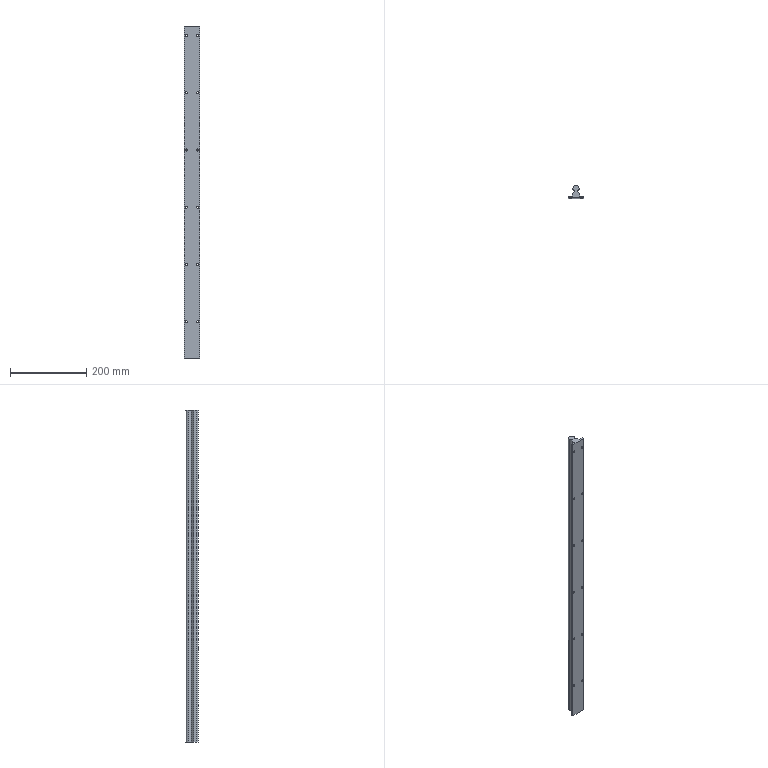Part | SolidWorks | features Extrusion 1, HoleWzd 1, ICE 1, LPattern 1 | 1 solid | 42 faces | box 40 x 33 x 870 mm | volume 521685 mm3 | cylinder 27 | plane 15 | commonest cylinder face diameters 5.5 x24 16 x3
STEP:
#1=CARTESIAN_POINT('',(15.,0.,-342.75));
#2=VERTEX_POINT('',#1);
#3=CARTESIAN_POINT('',(15.,0.,-337.25));
#4=VERTEX_POINT('',#3);
#5=CARTESIAN_POINT('',(15.,0.,-340.));
#6=DIRECTION('',(0.,1.,0.));
#7=DIRECTION('',(0.,0.,1.));
#8=AXIS2_PLACEMENT_3D('',#5,#6,#7);
#9=CIRCLE('',#8,2.75);
#10=EDGE_CURVE('',#2,#4,#9,.T.);
#11=ORIENTED_EDGE('',*,*,#10,.F.);
#12=CARTESIAN_POINT('',(15.,5.,-342.75));
#13=VERTEX_POINT('',#12);
#14=CARTESIAN_POINT('',(15.,5.,-342.75));
#15=DIRECTION('',(0.,1.,0.));
#16=VECTOR('',#15,1000.);
#17=LINE('',#14,#16);
#18=EDGE_CURVE('',#2,#13,#17,.T.);
#19=ORIENTED_EDGE('',*,*,#18,.T.);
#20=CARTESIAN_POINT('',(15.,5.,-337.25));
#21=VERTEX_POINT('',#20);
#22=CARTESIAN_POINT('',(15.,5.,-340.));
#23=DIRECTION('',(0.,1.,0.));
#24=DIRECTION('',(0.,0.,1.));
#25=AXIS2_PLACEMENT_3D('',#22,#23,#24);
#26=CIRCLE('',#25,2.75);
#27=EDGE_CURVE('',#13,#21,#26,.T.);
#28=ORIENTED_EDGE('',*,*,#27,.T.);
#29=CARTESIAN_POINT('',(15.,5.,-337.25));
#30=DIRECTION('',(0.,1.,0.));
#31=VECTOR('',#30,1000.);
#32=LINE('',#29,#31);
#33=EDGE_CURVE('',#4,#21,#32,.T.);
#34=ORIENTED_EDGE('',*,*,#33,.F.);
#35=EDGE_LOOP('',(#11,#19,#28,#34));
#36=FACE_OUTER_BOUND('',#35,.T.);
#37=CARTESIAN_POINT('',(15.,5.,-340.));
#38=DIRECTION('',(0.,1.,0.));
#39=DIRECTION('',(0.,0.,1.));
#40=AXIS2_PLACEMENT_3D('',#37,#38,#39);
#41=CYLINDRICAL_SURFACE('',#40,2.75);
#42=ADVANCED_FACE('',(#36),#41,.F.);
#43=CARTESIAN_POINT('',(-15.,0.,-342.75));
#44=VERTEX_POINT('',#43);
#45=CARTESIAN_POINT('',(-15.,0.,-337.25));
#46=VERTEX_POINT('',#45);
#47=CARTESIAN_POINT('',(-15.,0.,-340.));
#48=DIRECTION('',(0.,1.,0.));
#49=DIRECTION('',(0.,0.,1.));
#50=AXIS2_PLACEMENT_3D('',#47,#48,#49);
#51=CIRCLE('',#50,2.75);
#52=EDGE_CURVE('',#44,#46,#51,.T.);
#53=ORIENTED_EDGE('',*,*,#52,.F.);
#54=CARTESIAN_POINT('',(-15.,5.,-342.75));
#55=VERTEX_POINT('',#54);
#56=CARTESIAN_POINT('',(-15.,5.,-342.75));
#57=DIRECTION('',(0.,1.,0.));
#58=VECTOR('',#57,1000.);
#59=LINE('',#56,#58);
#60=EDGE_CURVE('',#44,#55,#59,.T.);
#61=ORIENTED_EDGE('',*,*,#60,.T.);
#62=CARTESIAN_POINT('',(-15.,5.,-337.25));
#63=VERTEX_POINT('',#62);
#64=CARTESIAN_POINT('',(-15.,5.,-340.));
#65=DIRECTION('',(0.,1.,0.));
#66=DIRECTION('',(0.,0.,1.));
#67=AXIS2_PLACEMENT_3D('',#64,#65,#66);
#68=CIRCLE('',#67,2.75);
#69=EDGE_CURVE('',#55,#63,#68,.T.);
#70=ORIENTED_EDGE('',*,*,#69,.T.);
#71=CARTESIAN_POINT('',(-15.,5.,-337.25));
#72=DIRECTION('',(0.,1.,0.));
#73=VECTOR('',#72,1000.);
#74=LINE('',#71,#73);
#75=EDGE_CURVE('',#46,#63,#74,.T.);
#76=ORIENTED_EDGE('',*,*,#75,.F.);
#77=EDGE_LOOP('',(#53,#61,#70,#76));
#78=FACE_OUTER_BOUND('',#77,.T.);
#79=CARTESIAN_POINT('',(-15.,5.,-340.));
#80=DIRECTION('',(0.,1.,0.));
#81=DIRECTION('',(0.,0.,1.));
#82=AXIS2_PLACEMENT_3D('',#79,#80,#81);
#83=CYLINDRICAL_SURFACE('',#82,2.75);
#84=ADVANCED_FACE('',(#78),#83,.F.);
#85=CARTESIAN_POINT('',(15.,0.,-192.75));
#86=VERTEX_POINT('',#85);
#87=CARTESIAN_POINT('',(15.,0.,-187.25));
#88=VERTEX_POINT('',#87);
#89=CARTESIAN_POINT('',(15.,0.,-190.));
#90=DIRECTION('',(0.,1.,0.));
#91=DIRECTION('',(0.,0.,1.));
#92=AXIS2_PLACEMENT_3D('',#89,#90,#91);
#93=CIRCLE('',#92,2.75);
#94=EDGE_CURVE('',#86,#88,#93,.T.);
#95=ORIENTED_EDGE('',*,*,#94,.F.);
#96=CARTESIAN_POINT('',(15.,5.,-192.75));
#97=VERTEX_POINT('',#96);
#98=CARTESIAN_POINT('',(15.,5.,-192.75));
#99=DIRECTION('',(0.,1.,0.));
#100=VECTOR('',#99,1000.);
#101=LINE('',#98,#100);
#102=EDGE_CURVE('',#86,#97,#101,.T.);
#103=ORIENTED_EDGE('',*,*,#102,.T.);
#104=CARTESIAN_POINT('',(15.,5.,-187.25));
#105=VERTEX_POINT('',#104);
#106=CARTESIAN_POINT('',(15.,5.,-190.));
#107=DIRECTION('',(0.,1.,0.));
#108=DIRECTION('',(0.,0.,1.));
#109=AXIS2_PLACEMENT_3D('',#106,#107,#108);
#110=CIRCLE('',#109,2.75);
#111=EDGE_CURVE('',#97,#105,#110,.T.);
#112=ORIENTED_EDGE('',*,*,#111,.T.);
#113=CARTESIAN_POINT('',(15.,5.,-187.25));
#114=DIRECTION('',(0.,1.,0.));
#115=VECTOR('',#114,1000.);
#116=LINE('',#113,#115);
#117=EDGE_CURVE('',#88,#105,#116,.T.);
#118=ORIENTED_EDGE('',*,*,#117,.F.);
#119=EDGE_LOOP('',(#95,#103,#112,#118));
#120=FACE_OUTER_BOUND('',#119,.T.);
#121=CARTESIAN_POINT('',(15.,5.,-190.));
#122=DIRECTION('',(0.,1.,0.));
#123=DIRECTION('',(0.,0.,1.));
#124=AXIS2_PLACEMENT_3D('',#121,#122,#123);
#125=CYLINDRICAL_SURFACE('',#124,2.75);
#126=ADVANCED_FACE('',(#120),#125,.F.);
#127=CARTESIAN_POINT('',(-15.,0.,-192.75));
#128=VERTEX_POINT('',#127);
#129=CARTESIAN_POINT('',(-15.,0.,-187.25));
#130=VERTEX_POINT('',#129);
#131=CARTESIAN_POINT('',(-15.,0.,-190.));
#132=DIRECTION('',(0.,1.,0.));
#133=DIRECTION('',(0.,0.,1.));
#134=AXIS2_PLACEMENT_3D('',#131,#132,#133);
#135=CIRCLE('',#134,2.75);
#136=EDGE_CURVE('',#128,#130,#135,.T.);
#137=ORIENTED_EDGE('',*,*,#136,.F.);
#138=CARTESIAN_POINT('',(-15.,5.,-192.75));
#139=VERTEX_POINT('',#138);
#140=CARTESIAN_POINT('',(-15.,5.,-192.75));
#141=DIRECTION('',(0.,1.,0.));
#142=VECTOR('',#141,1000.);
#143=LINE('',#140,#142);
#144=EDGE_CURVE('',#128,#139,#143,.T.);
#145=ORIENTED_EDGE('',*,*,#144,.T.);
#146=CARTESIAN_POINT('',(-15.,5.,-187.25));
#147=VERTEX_POINT('',#146);
#148=CARTESIAN_POINT('',(-15.,5.,-190.));
#149=DIRECTION('',(0.,1.,0.));
#150=DIRECTION('',(0.,0.,1.));
#151=AXIS2_PLACEMENT_3D('',#148,#149,#150);
#152=CIRCLE('',#151,2.75);
#153=EDGE_CURVE('',#139,#147,#152,.T.);
#154=ORIENTED_EDGE('',*,*,#153,.T.);
#155=CARTESIAN_POINT('',(-15.,5.,-187.25));
#156=DIRECTION('',(0.,1.,0.));
#157=VECTOR('',#156,1000.);
#158=LINE('',#155,#157);
#159=EDGE_CURVE('',#130,#147,#158,.T.);
#160=ORIENTED_EDGE('',*,*,#159,.F.);
#161=EDGE_LOOP('',(#137,#145,#154,#160));
#162=FACE_OUTER_BOUND('',#161,.T.);
#163=CARTESIAN_POINT('',(-15.,5.,-190.));
#164=DIRECTION('',(0.,1.,0.));
#165=DIRECTION('',(0.,0.,1.));
#166=AXIS2_PLACEMENT_3D('',#163,#164,#165);
#167=CYLINDRICAL_SURFACE('',#166,2.75);
#168=ADVANCED_FACE('',(#162),#167,.F.);
#169=CARTESIAN_POINT('',(15.,0.,-42.75));
#170=VERTEX_POINT('',#169);
#171=CARTESIAN_POINT('',(15.,0.,-37.25));
#172=VERTEX_POINT('',#171);
#173=CARTESIAN_POINT('',(15.,0.,-40.));
#174=DIRECTION('',(0.,1.,0.));
#175=DIRECTION('',(0.,0.,1.));
#176=AXIS2_PLACEMENT_3D('',#173,#174,#175);
#177=CIRCLE('',#176,2.75);
#178=EDGE_CURVE('',#170,#172,#177,.T.);
#179=ORIENTED_EDGE('',*,*,#178,.F.);
#180=CARTESIAN_POINT('',(15.,5.,-42.75));
#181=VERTEX_POINT('',#180);
#182=CARTESIAN_POINT('',(15.,5.,-42.75));
#183=DIRECTION('',(0.,1.,0.));
#184=VECTOR('',#183,1000.);
#185=LINE('',#182,#184);
#186=EDGE_CURVE('',#170,#181,#185,.T.);
#187=ORIENTED_EDGE('',*,*,#186,.T.);
#188=CARTESIAN_POINT('',(15.,5.,-37.25));
#189=VERTEX_POINT('',#188);
#190=CARTESIAN_POINT('',(15.,5.,-40.));
#191=DIRECTION('',(0.,1.,0.));
#192=DIRECTION('',(0.,0.,1.));
#193=AXIS2_PLACEMENT_3D('',#190,#191,#192);
#194=CIRCLE('',#193,2.75);
#195=EDGE_CURVE('',#181,#189,#194,.T.);
#196=ORIENTED_EDGE('',*,*,#195,.T.);
#197=CARTESIAN_POINT('',(15.,5.,-37.25));
#198=DIRECTION('',(0.,1.,0.));
#199=VECTOR('',#198,1000.);
#200=LINE('',#197,#199);
#201=EDGE_CURVE('',#172,#189,#200,.T.);
#202=ORIENTED_EDGE('',*,*,#201,.F.);
#203=EDGE_LOOP('',(#179,#187,#196,#202));
#204=FACE_OUTER_BOUND('',#203,.T.);
#205=CARTESIAN_POINT('',(15.,5.,-40.));
#206=DIRECTION('',(0.,1.,0.));
#207=DIRECTION('',(0.,0.,1.));
#208=AXIS2_PLACEMENT_3D('',#205,#206,#207);
#209=CYLINDRICAL_SURFACE('',#208,2.75);
#210=ADVANCED_FACE('',(#204),#209,.F.);
#211=CARTESIAN_POINT('',(-15.,0.,-42.75));
#212=VERTEX_POINT('',#211);
#213=CARTESIAN_POINT('',(-15.,0.,-37.25));
#214=VERTEX_POINT('',#213);
#215=CARTESIAN_POINT('',(-15.,0.,-40.));
#216=DIRECTION('',(0.,1.,0.));
#217=DIRECTION('',(0.,0.,1.));
#218=AXIS2_PLACEMENT_3D('',#215,#216,#217);
#219=CIRCLE('',#218,2.75);
#220=EDGE_CURVE('',#212,#214,#219,.T.);
#221=ORIENTED_EDGE('',*,*,#220,.F.);
#222=CARTESIAN_POINT('',(-15.,5.,-42.75));
#223=VERTEX_POINT('',#222);
#224=CARTESIAN_POINT('',(-15.,5.,-42.75));
#225=DIRECTION('',(0.,1.,0.));
#226=VECTOR('',#225,1000.);
#227=LINE('',#224,#226);
#228=EDGE_CURVE('',#212,#223,#227,.T.);
#229=ORIENTED_EDGE('',*,*,#228,.T.);
#230=CARTESIAN_POINT('',(-15.,5.,-37.25));
#231=VERTEX_POINT('',#230);
#232=CARTESIAN_POINT('',(-15.,5.,-40.));
#233=DIRECTION('',(0.,1.,0.));
#234=DIRECTION('',(0.,0.,1.));
#235=AXIS2_PLACEMENT_3D('',#232,#233,#234);
#236=CIRCLE('',#235,2.75);
#237=EDGE_CURVE('',#223,#231,#236,.T.);
#238=ORIENTED_EDGE('',*,*,#237,.T.);
#239=CARTESIAN_POINT('',(-15.,5.,-37.25));
#240=DIRECTION('',(0.,1.,0.));
#241=VECTOR('',#240,1000.);
#242=LINE('',#239,#241);
#243=EDGE_CURVE('',#214,#231,#242,.T.);
#244=ORIENTED_EDGE('',*,*,#243,.F.);
#245=EDGE_LOOP('',(#221,#229,#238,#244));
#246=FACE_OUTER_BOUND('',#245,.T.);
#247=CARTESIAN_POINT('',(-15.,5.,-40.));
#248=DIRECTION('',(0.,1.,0.));
#249=DIRECTION('',(0.,0.,1.));
#250=AXIS2_PLACEMENT_3D('',#247,#248,#249);
#251=CYLINDRICAL_SURFACE('',#250,2.75);
#252=ADVANCED_FACE('',(#246),#251,.F.);
#253=CARTESIAN_POINT('',(15.,0.,107.25));
#254=VERTEX_POINT('',#253);
#255=CARTESIAN_POINT('',(15.,0.,112.75));
#256=VERTEX_POINT('',#255);
#257=CARTESIAN_POINT('',(15.,0.,110.));
#258=DIRECTION('',(0.,1.,0.));
#259=DIRECTION('',(0.,0.,1.));
#260=AXIS2_PLACEMENT_3D('',#257,#258,#259);
#261=CIRCLE('',#260,2.75);
#262=EDGE_CURVE('',#254,#256,#261,.T.);
#263=ORIENTED_EDGE('',*,*,#262,.F.);
#264=CARTESIAN_POINT('',(15.,5.,107.25));
#265=VERTEX_POINT('',#264);
#266=CARTESIAN_POINT('',(15.,5.,107.25));
#267=DIRECTION('',(0.,1.,0.));
#268=VECTOR('',#267,1000.);
#269=LINE('',#266,#268);
#270=EDGE_CURVE('',#254,#265,#269,.T.);
#271=ORIENTED_EDGE('',*,*,#270,.T.);
#272=CARTESIAN_POINT('',(15.,5.,112.75));
#273=VERTEX_POINT('',#272);
#274=CARTESIAN_POINT('',(15.,5.,110.));
#275=DIRECTION('',(0.,1.,0.));
#276=DIRECTION('',(0.,0.,1.));
#277=AXIS2_PLACEMENT_3D('',#274,#275,#276);
#278=CIRCLE('',#277,2.75);
#279=EDGE_CURVE('',#265,#273,#278,.T.);
#280=ORIENTED_EDGE('',*,*,#279,.T.);
#281=CARTESIAN_POINT('',(15.,5.,112.75));
#282=DIRECTION('',(0.,1.,0.));
#283=VECTOR('',#282,1000.);
#284=LINE('',#281,#283);
#285=EDGE_CURVE('',#256,#273,#284,.T.);
#286=ORIENTED_EDGE('',*,*,#285,.F.);
#287=EDGE_LOOP('',(#263,#271,#280,#286));
#288=FACE_OUTER_BOUND('',#287,.T.);
#289=CARTESIAN_POINT('',(15.,5.,110.));
#290=DIRECTION('',(0.,1.,0.));
#291=DIRECTION('',(0.,0.,1.));
#292=AXIS2_PLACEMENT_3D('',#289,#290,#291);
#293=CYLINDRICAL_SURFACE('',#292,2.75);
#294=ADVANCED_FACE('',(#288),#293,.F.);
#295=CARTESIAN_POINT('',(-15.,0.,107.25));
#296=VERTEX_POINT('',#295);
#297=CARTESIAN_POINT('',(-15.,0.,112.75));
#298=VERTEX_POINT('',#297);
#299=CARTESIAN_POINT('',(-15.,0.,110.));
#300=DIRECTION('',(0.,1.,0.));
#301=DIRECTION('',(0.,0.,1.));
#302=AXIS2_PLACEMENT_3D('',#299,#300,#301);
#303=CIRCLE('',#302,2.75);
#304=EDGE_CURVE('',#296,#298,#303,.T.);
#305=ORIENTED_EDGE('',*,*,#304,.F.);
#306=CARTESIAN_POINT('',(-15.,5.,107.25));
#307=VERTEX_POINT('',#306);
#308=CARTESIAN_POINT('',(-15.,5.,107.25));
#309=DIRECTION('',(0.,1.,0.));
#310=VECTOR('',#309,1000.);
#311=LINE('',#308,#310);
#312=EDGE_CURVE('',#296,#307,#311,.T.);
#313=ORIENTED_EDGE('',*,*,#312,.T.);
#314=CARTESIAN_POINT('',(-15.,5.,112.75));
#315=VERTEX_POINT('',#314);
#316=CARTESIAN_POINT('',(-15.,5.,110.));
#317=DIRECTION('',(0.,1.,0.));
#318=DIRECTION('',(0.,0.,1.));
#319=AXIS2_PLACEMENT_3D('',#316,#317,#318);
#320=CIRCLE('',#319,2.75);
#321=EDGE_CURVE('',#307,#315,#320,.T.);
#322=ORIENTED_EDGE('',*,*,#321,.T.);
#323=CARTESIAN_POINT('',(-15.,5.,112.75));
#324=DIRECTION('',(0.,1.,0.));
#325=VECTOR('',#324,1000.);
#326=LINE('',#323,#325);
#327=EDGE_CURVE('',#298,#315,#326,.T.);
#328=ORIENTED_EDGE('',*,*,#327,.F.);
#329=EDGE_LOOP('',(#305,#313,#322,#328));
#330=FACE_OUTER_BOUND('',#329,.T.);
#331=CARTESIAN_POINT('',(-15.,5.,110.));
#332=DIRECTION('',(0.,1.,0.));
#333=DIRECTION('',(0.,0.,1.));
#334=AXIS2_PLACEMENT_3D('',#331,#332,#333);
#335=CYLINDRICAL_SURFACE('',#334,2.75);
#336=ADVANCED_FACE('',(#330),#335,.F.);
#337=CARTESIAN_POINT('',(15.,0.,257.25));
#338=VERTEX_POINT('',#337);
#339=CARTESIAN_POINT('',(15.,0.,262.75));
#340=VERTEX_POINT('',#339);
#341=CARTESIAN_POINT('',(15.,0.,260.));
#342=DIRECTION('',(0.,1.,0.));
#343=DIRECTION('',(0.,0.,1.));
#344=AXIS2_PLACEMENT_3D('',#341,#342,#343);
#345=CIRCLE('',#344,2.75);
#346=EDGE_CURVE('',#338,#340,#345,.T.);
#347=ORIENTED_EDGE('',*,*,#346,.F.);
#348=CARTESIAN_POINT('',(15.,5.,257.25));
#349=VERTEX_POINT('',#348);
#350=CARTESIAN_POINT('',(15.,5.,257.25));
#351=DIRECTION('',(0.,1.,0.));
#352=VECTOR('',#351,1000.);
#353=LINE('',#350,#352);
#354=EDGE_CURVE('',#338,#349,#353,.T.);
#355=ORIENTED_EDGE('',*,*,#354,.T.);
#356=CARTESIAN_POINT('',(15.,5.,262.75));
#357=VERTEX_POINT('',#356);
#358=CARTESIAN_POINT('',(15.,5.,260.));
#359=DIRECTION('',(0.,1.,0.));
#360=DIRECTION('',(0.,0.,1.));
#361=AXIS2_PLACEMENT_3D('',#358,#359,#360);
#362=CIRCLE('',#361,2.75);
#363=EDGE_CURVE('',#349,#357,#362,.T.);
#364=ORIENTED_EDGE('',*,*,#363,.T.);
#365=CARTESIAN_POINT('',(15.,5.,262.75));
#366=DIRECTION('',(0.,1.,0.));
#367=VECTOR('',#366,1000.);
#368=LINE('',#365,#367);
#369=EDGE_CURVE('',#340,#357,#368,.T.);
#370=ORIENTED_EDGE('',*,*,#369,.F.);
#371=EDGE_LOOP('',(#347,#355,#364,#370));
#372=FACE_OUTER_BOUND('',#371,.T.);
#373=CARTESIAN_POINT('',(15.,5.,260.));
#374=DIRECTION('',(0.,1.,0.));
#375=DIRECTION('',(0.,0.,1.));
#376=AXIS2_PLACEMENT_3D('',#373,#374,#375);
#377=CYLINDRICAL_SURFACE('',#376,2.75);
#378=ADVANCED_FACE('',(#372),#377,.F.);
#379=CARTESIAN_POINT('',(-15.,0.,257.25));
#380=VERTEX_POINT('',#379);
#381=CARTESIAN_POINT('',(-15.,0.,262.75));
#382=VERTEX_POINT('',#381);
#383=CARTESIAN_POINT('',(-15.,0.,260.));
#384=DIRECTION('',(0.,1.,0.));
#385=DIRECTION('',(0.,0.,1.));
#386=AXIS2_PLACEMENT_3D('',#383,#384,#385);
#387=CIRCLE('',#386,2.75);
#388=EDGE_CURVE('',#380,#382,#387,.T.);
#389=ORIENTED_EDGE('',*,*,#388,.F.);
#390=CARTESIAN_POINT('',(-15.,5.,257.25));
#391=VERTEX_POINT('',#390);
#392=CARTESIAN_POINT('',(-15.,5.,257.25));
#393=DIRECTION('',(0.,1.,0.));
#394=VECTOR('',#393,1000.);
#395=LINE('',#392,#394);
#396=EDGE_CURVE('',#380,#391,#395,.T.);
#397=ORIENTED_EDGE('',*,*,#396,.T.);
#398=CARTESIAN_POINT('',(-15.,5.,262.75));
#399=VERTEX_POINT('',#398);
#400=CARTESIAN_POINT('',(-15.,5.,260.));
#401=DIRECTION('',(0.,1.,0.));
#402=DIRECTION('',(0.,0.,1.));
#403=AXIS2_PLACEMENT_3D('',#400,#401,#402);
#404=CIRCLE('',#403,2.75);
#405=EDGE_CURVE('',#391,#399,#404,.T.);
#406=ORIENTED_EDGE('',*,*,#405,.T.);
#407=CARTESIAN_POINT('',(-15.,5.,262.75));
#408=DIRECTION('',(0.,1.,0.));
#409=VECTOR('',#408,1000.);
#410=LINE('',#407,#409);
#411=EDGE_CURVE('',#382,#399,#410,.T.);
#412=ORIENTED_EDGE('',*,*,#411,.F.);
#413=EDGE_LOOP('',(#389,#397,#406,#412));
#414=FACE_OUTER_BOUND('',#413,.T.);
#415=CARTESIAN_POINT('',(-15.,5.,260.));
#416=DIRECTION('',(0.,1.,0.));
#417=DIRECTION('',(0.,0.,1.));
#418=AXIS2_PLACEMENT_3D('',#415,#416,#417);
#419=CYLINDRICAL_SURFACE('',#418,2.75);
#420=ADVANCED_FACE('',(#414),#419,.F.);
#421=CARTESIAN_POINT('',(15.,0.,407.25));
#422=VERTEX_POINT('',#421);
#423=CARTESIAN_POINT('',(15.,0.,412.75));
#424=VERTEX_POINT('',#423);
#425=CARTESIAN_POINT('',(15.,0.,410.));
#426=DIRECTION('',(0.,1.,0.));
#427=DIRECTION('',(0.,0.,1.));
#428=AXIS2_PLACEMENT_3D('',#425,#426,#427);
#429=CIRCLE('',#428,2.75);
#430=EDGE_CURVE('',#422,#424,#429,.T.);
#431=ORIENTED_EDGE('',*,*,#430,.F.);
#432=CARTESIAN_POINT('',(15.,5.,407.25));
#433=VERTEX_POINT('',#432);
#434=CARTESIAN_POINT('',(15.,5.,407.25));
#435=DIRECTION('',(0.,1.,0.));
#436=VECTOR('',#435,1000.);
#437=LINE('',#434,#436);
#438=EDGE_CURVE('',#422,#433,#437,.T.);
#439=ORIENTED_EDGE('',*,*,#438,.T.);
#440=CARTESIAN_POINT('',(15.,5.,412.75));
#441=VERTEX_POINT('',#440);
#442=CARTESIAN_POINT('',(15.,5.,410.));
#443=DIRECTION('',(0.,1.,0.));
#444=DIRECTION('',(0.,0.,1.));
#445=AXIS2_PLACEMENT_3D('',#442,#443,#444);
#446=CIRCLE('',#445,2.75);
#447=EDGE_CURVE('',#433,#441,#446,.T.);
#448=ORIENTED_EDGE('',*,*,#447,.T.);
#449=CARTESIAN_POINT('',(15.,5.,412.75));
#450=DIRECTION('',(0.,1.,0.));
#451=VECTOR('',#450,1000.);
#452=LINE('',#449,#451);
#453=EDGE_CURVE('',#424,#441,#452,.T.);
#454=ORIENTED_EDGE('',*,*,#453,.F.);
#455=EDGE_LOOP('',(#431,#439,#448,#454));
#456=FACE_OUTER_BOUND('',#455,.T.);
#457=CARTESIAN_POINT('',(15.,5.,410.));
#458=DIRECTION('',(0.,1.,0.));
#459=DIRECTION('',(0.,0.,1.));
#460=AXIS2_PLACEMENT_3D('',#457,#458,#459);
#461=CYLINDRICAL_SURFACE('',#460,2.75);
#462=ADVANCED_FACE('',(#456),#461,.F.);
#463=CARTESIAN_POINT('',(-15.,0.,407.25));
#464=VERTEX_POINT('',#463);
#465=CARTESIAN_POINT('',(-15.,0.,412.75));
#466=VERTEX_POINT('',#465);
#467=CARTESIAN_POINT('',(-15.,0.,410.));
#468=DIRECTION('',(0.,1.,0.));
#469=DIRECTION('',(0.,0.,1.));
#470=AXIS2_PLACEMENT_3D('',#467,#468,#469);
#471=CIRCLE('',#470,2.75);
#472=EDGE_CURVE('',#464,#466,#471,.T.);
#473=ORIENTED_EDGE('',*,*,#472,.F.);
#474=CARTESIAN_POINT('',(-15.,5.,407.25));
#475=VERTEX_POINT('',#474);
#476=CARTESIAN_POINT('',(-15.,5.,407.25));
#477=DIRECTION('',(0.,1.,0.));
#478=VECTOR('',#477,1000.);
#479=LINE('',#476,#478);
#480=EDGE_CURVE('',#464,#475,#479,.T.);
#481=ORIENTED_EDGE('',*,*,#480,.T.);
#482=CARTESIAN_POINT('',(-15.,5.,412.75));
#483=VERTEX_POINT('',#482);
#484=CARTESIAN_POINT('',(-15.,5.,410.));
#485=DIRECTION('',(0.,1.,0.));
#486=DIRECTION('',(0.,0.,1.));
#487=AXIS2_PLACEMENT_3D('',#484,#485,#486);
#488=CIRCLE('',#487,2.75);
#489=EDGE_CURVE('',#475,#483,#488,.T.);
#490=ORIENTED_EDGE('',*,*,#489,.T.);
#491=CARTESIAN_POINT('',(-15.,5.,412.75));
#492=DIRECTION('',(0.,1.,0.));
#493=VECTOR('',#492,1000.);
#494=LINE('',#491,#493);
#495=EDGE_CURVE('',#466,#483,#494,.T.);
#496=ORIENTED_EDGE('',*,*,#495,.F.);
#497=EDGE_LOOP('',(#473,#481,#490,#496));
#498=FACE_OUTER_BOUND('',#497,.T.);
#499=CARTESIAN_POINT('',(-15.,5.,410.));
#500=DIRECTION('',(0.,1.,0.));
#501=DIRECTION('',(0.,0.,1.));
#502=AXIS2_PLACEMENT_3D('',#499,#500,#501);
#503=CYLINDRICAL_SURFACE('',#502,2.75);
#504=ADVANCED_FACE('',(#498),#503,.F.);
#505=CARTESIAN_POINT('',(-8.,25.,-435.));
#506=VERTEX_POINT('',#505);
#507=CARTESIAN_POINT('',(8.,25.,-435.));
#508=VERTEX_POINT('',#507);
#509=CARTESIAN_POINT('',(0.,25.,-435.));
#510=DIRECTION('',(0.,0.,-1.));
#511=DIRECTION('',(1.,0.,0.));
#512=AXIS2_PLACEMENT_3D('',#509,#510,#511);
#513=CIRCLE('',#512,8.);
#514=EDGE_CURVE('',#506,#508,#513,.T.);
#515=ORIENTED_EDGE('',*,*,#514,.F.);
#516=CARTESIAN_POINT('',(-8.,25.,435.));
#517=VERTEX_POINT('',#516);
#518=CARTESIAN_POINT('',(-8.,25.,-457.627));
#519=DIRECTION('',(0.,0.,1.));
#520=VECTOR('',#519,1000.);
#521=LINE('',#518,#520);
#522=EDGE_CURVE('',#506,#517,#521,.T.);
#523=ORIENTED_EDGE('',*,*,#522,.T.);
#524=CARTESIAN_POINT('',(8.,25.,435.));
#525=VERTEX_POINT('',#524);
#526=CARTESIAN_POINT('',(0.,25.,435.));
#527=DIRECTION('',(0.,0.,1.));
#528=DIRECTION('',(1.,0.,0.));
#529=AXIS2_PLACEMENT_3D('',#526,#527,#528);
#530=CIRCLE('',#529,8.);
#531=EDGE_CURVE('',#525,#517,#530,.T.);
#532=ORIENTED_EDGE('',*,*,#531,.F.);
#533=CARTESIAN_POINT('',(8.,25.,-457.627));
#534=DIRECTION('',(0.,0.,1.));
#535=VECTOR('',#534,1000.);
#536=LINE('',#533,#535);
#537=EDGE_CURVE('',#508,#525,#536,.T.);
#538=ORIENTED_EDGE('',*,*,#537,.F.);
#539=EDGE_LOOP('',(#515,#523,#532,#538));
#540=FACE_OUTER_BOUND('',#539,.T.);
#541=CARTESIAN_POINT('',(0.,25.,-457.627));
#542=DIRECTION('',(0.,0.,1.));
#543=DIRECTION('',(1.,0.,0.));
#544=AXIS2_PLACEMENT_3D('',#541,#542,#543);
#545=CYLINDRICAL_SURFACE('',#544,8.);
#546=ADVANCED_FACE('',(#540),#545,.T.);
#547=CARTESIAN_POINT('',(3.487,17.8,-435.));
#548=VERTEX_POINT('',#547);
#549=CARTESIAN_POINT('',(0.,25.,-435.));
#550=DIRECTION('',(0.,0.,-1.));
#551=DIRECTION('',(1.,0.,0.));
#552=AXIS2_PLACEMENT_3D('',#549,#550,#551);
#553=CIRCLE('',#552,8.);
#554=EDGE_CURVE('',#508,#548,#553,.T.);
#555=ORIENTED_EDGE('',*,*,#554,.F.);
#556=ORIENTED_EDGE('',*,*,#537,.T.);
#557=CARTESIAN_POINT('',(3.487,17.8,435.));
#558=VERTEX_POINT('',#557);
#559=CARTESIAN_POINT('',(0.,25.,435.));
#560=DIRECTION('',(0.,0.,1.));
#561=DIRECTION('',(1.,0.,0.));
#562=AXIS2_PLACEMENT_3D('',#559,#560,#561);
#563=CIRCLE('',#562,8.);
#564=EDGE_CURVE('',#558,#525,#563,.T.);
#565=ORIENTED_EDGE('',*,*,#564,.F.);
#566=CARTESIAN_POINT('',(3.487,17.8,435.));
#567=DIRECTION('',(0.,0.,-1.));
#568=VECTOR('',#567,1000.);
#569=LINE('',#566,#568);
#570=EDGE_CURVE('',#558,#548,#569,.T.);
#571=ORIENTED_EDGE('',*,*,#570,.T.);
#572=EDGE_LOOP('',(#555,#556,#565,#571));
#573=FACE_OUTER_BOUND('',#572,.T.);
#574=CARTESIAN_POINT('',(0.,25.,-457.627));
#575=DIRECTION('',(0.,0.,1.));
#576=DIRECTION('',(1.,0.,0.));
#577=AXIS2_PLACEMENT_3D('',#574,#575,#576);
#578=CYLINDRICAL_SURFACE('',#577,8.);
#579=ADVANCED_FACE('',(#573),#578,.T.);
#580=CARTESIAN_POINT('',(15.,5.,-340.));
#581=DIRECTION('',(0.,1.,0.));
#582=DIRECTION('',(0.,0.,1.));
#583=AXIS2_PLACEMENT_3D('',#580,#581,#582);
#584=CIRCLE('',#583,2.75);
#585=EDGE_CURVE('',#21,#13,#584,.T.);
#586=ORIENTED_EDGE('',*,*,#585,.F.);
#587=ORIENTED_EDGE('',*,*,#27,.F.);
#588=EDGE_LOOP('',(#586,#587));
#589=FACE_BOUND('',#588,.T.);
#590=CARTESIAN_POINT('',(15.,5.,-190.));
#591=DIRECTION('',(0.,1.,0.));
#592=DIRECTION('',(0.,0.,1.));
#593=AXIS2_PLACEMENT_3D('',#590,#591,#592);
#594=CIRCLE('',#593,2.75);
#595=EDGE_CURVE('',#105,#97,#594,.T.);
#596=ORIENTED_EDGE('',*,*,#595,.F.);
#597=ORIENTED_EDGE('',*,*,#111,.F.);
#598=EDGE_LOOP('',(#596,#597));
#599=FACE_BOUND('',#598,.T.);
#600=CARTESIAN_POINT('',(15.,5.,-40.));
#601=DIRECTION('',(0.,1.,0.));
#602=DIRECTION('',(0.,0.,1.));
#603=AXIS2_PLACEMENT_3D('',#600,#601,#602);
#604=CIRCLE('',#603,2.75);
#605=EDGE_CURVE('',#189,#181,#604,.T.);
#606=ORIENTED_EDGE('',*,*,#605,.F.);
#607=ORIENTED_EDGE('',*,*,#195,.F.);
#608=EDGE_LOOP('',(#606,#607));
#609=FACE_BOUND('',#608,.T.);
#610=CARTESIAN_POINT('',(20.,5.,-435.));
#611=VERTEX_POINT('',#610);
#612=CARTESIAN_POINT('',(9.25,5.,-435.));
#613=VERTEX_POINT('',#612);
#614=CARTESIAN_POINT('',(20.,5.,-435.));
#615=DIRECTION('',(-1.,0.,0.));
#616=VECTOR('',#615,1000.);
#617=LINE('',#614,#616);
#618=EDGE_CURVE('',#611,#613,#617,.T.);
#619=ORIENTED_EDGE('',*,*,#618,.T.);
#620=CARTESIAN_POINT('',(9.25,5.,435.));
#621=VERTEX_POINT('',#620);
#622=CARTESIAN_POINT('',(9.25,5.,435.));
#623=DIRECTION('',(0.,0.,-1.));
#624=VECTOR('',#623,1000.);
#625=LINE('',#622,#624);
#626=EDGE_CURVE('',#621,#613,#625,.T.);
#627=ORIENTED_EDGE('',*,*,#626,.F.);
#628=CARTESIAN_POINT('',(20.,5.,435.));
#629=VERTEX_POINT('',#628);
#630=CARTESIAN_POINT('',(20.,5.,435.));
#631=DIRECTION('',(-1.,0.,0.));
#632=VECTOR('',#631,1000.);
#633=LINE('',#630,#632);
#634=EDGE_CURVE('',#629,#621,#633,.T.);
#635=ORIENTED_EDGE('',*,*,#634,.F.);
#636=CARTESIAN_POINT('',(20.,5.,435.));
#637=DIRECTION('',(0.,0.,-1.));
#638=VECTOR('',#637,1000.);
#639=LINE('',#636,#638);
#640=EDGE_CURVE('',#629,#611,#639,.T.);
#641=ORIENTED_EDGE('',*,*,#640,.T.);
#642=EDGE_LOOP('',(#619,#627,#635,#641));
#643=FACE_OUTER_BOUND('',#642,.T.);
#644=CARTESIAN_POINT('',(15.,5.,410.));
#645=DIRECTION('',(0.,1.,0.));
#646=DIRECTION('',(0.,0.,1.));
#647=AXIS2_PLACEMENT_3D('',#644,#645,#646);
#648=CIRCLE('',#647,2.75);
#649=EDGE_CURVE('',#441,#433,#648,.T.);
#650=ORIENTED_EDGE('',*,*,#649,.F.);
#651=ORIENTED_EDGE('',*,*,#447,.F.);
#652=EDGE_LOOP('',(#650,#651));
#653=FACE_BOUND('',#652,.T.);
#654=CARTESIAN_POINT('',(15.,5.,260.));
#655=DIRECTION('',(0.,1.,0.));
#656=DIRECTION('',(0.,0.,1.));
#657=AXIS2_PLACEMENT_3D('',#654,#655,#656);
#658=CIRCLE('',#657,2.75);
#659=EDGE_CURVE('',#357,#349,#658,.T.);
#660=ORIENTED_EDGE('',*,*,#659,.F.);
#661=ORIENTED_EDGE('',*,*,#363,.F.);
#662=EDGE_LOOP('',(#660,#661));
#663=FACE_BOUND('',#662,.T.);
#664=CARTESIAN_POINT('',(15.,5.,110.));
#665=DIRECTION('',(0.,1.,0.));
#666=DIRECTION('',(0.,0.,1.));
#667=AXIS2_PLACEMENT_3D('',#664,#665,#666);
#668=CIRCLE('',#667,2.75);
#669=EDGE_CURVE('',#273,#265,#668,.T.);
#670=ORIENTED_EDGE('',*,*,#669,.F.);
#671=ORIENTED_EDGE('',*,*,#279,.F.);
#672=EDGE_LOOP('',(#670,#671));
#673=FACE_BOUND('',#672,.T.);
#674=CARTESIAN_POINT('',(20.,5.,435.));
#675=DIRECTION('',(0.,-1.,0.));
#676=DIRECTION('',(0.,0.,-1.));
#677=AXIS2_PLACEMENT_3D('',#674,#675,#676);
#678=PLANE('',#677);
#679=ADVANCED_FACE('',(#589,#599,#609,#643,#653,#663,#673),#678,.F.);
#680=CARTESIAN_POINT('',(-9.119,11.7,-435.));
#681=VERTEX_POINT('',#680);
#682=CARTESIAN_POINT('',(-9.25,11.7,-435.));
#683=VERTEX_POINT('',#682);
#684=CARTESIAN_POINT('',(-9.119,11.7,-435.));
#685=DIRECTION('',(-1.,0.,0.));
#686=VECTOR('',#685,1000.);
#687=LINE('',#684,#686);
#688=EDGE_CURVE('',#681,#683,#687,.T.);
#689=ORIENTED_EDGE('',*,*,#688,.T.);
#690=CARTESIAN_POINT('',(-9.25,11.7,435.));
#691=VERTEX_POINT('',#690);
#692=CARTESIAN_POINT('',(-9.25,11.7,435.));
#693=DIRECTION('',(0.,0.,-1.));
#694=VECTOR('',#693,1000.);
#695=LINE('',#692,#694);
#696=EDGE_CURVE('',#691,#683,#695,.T.);
#697=ORIENTED_EDGE('',*,*,#696,.F.);
#698=CARTESIAN_POINT('',(-9.119,11.7,435.));
#699=VERTEX_POINT('',#698);
#700=CARTESIAN_POINT('',(-9.119,11.7,435.));
#701=DIRECTION('',(-1.,0.,0.));
#702=VECTOR('',#701,1000.);
#703=LINE('',#700,#702);
#704=EDGE_CURVE('',#699,#691,#703,.T.);
#705=ORIENTED_EDGE('',*,*,#704,.F.);
#706=CARTESIAN_POINT('',(-9.119,11.7,435.));
#707=DIRECTION('',(0.,0.,-1.));
#708=VECTOR('',#707,1000.);
#709=LINE('',#706,#708);
#710=EDGE_CURVE('',#699,#681,#709,.T.);
#711=ORIENTED_EDGE('',*,*,#710,.T.);
#712=EDGE_LOOP('',(#689,#697,#705,#711));
#713=FACE_OUTER_BOUND('',#712,.T.);
#714=CARTESIAN_POINT('',(-9.119,11.7,435.));
#715=DIRECTION('',(0.,-1.,0.));
#716=DIRECTION('',(0.,0.,-1.));
#717=AXIS2_PLACEMENT_3D('',#714,#715,#716);
#718=PLANE('',#717);
#719=ADVANCED_FACE('',(#713),#718,.F.);
#720=CARTESIAN_POINT('',(-9.25,5.,-435.));
#721=VERTEX_POINT('',#720);
#722=CARTESIAN_POINT('',(-9.25,11.7,-435.));
#723=DIRECTION('',(0.,-1.,0.));
#724=VECTOR('',#723,1000.);
#725=LINE('',#722,#724);
#726=EDGE_CURVE('',#683,#721,#725,.T.);
#727=ORIENTED_EDGE('',*,*,#726,.T.);
#728=CARTESIAN_POINT('',(-9.25,5.,435.));
#729=VERTEX_POINT('',#728);
#730=CARTESIAN_POINT('',(-9.25,5.,435.));
#731=DIRECTION('',(0.,0.,-1.));
#732=VECTOR('',#731,1000.);
#733=LINE('',#730,#732);
#734=EDGE_CURVE('',#729,#721,#733,.T.);
#735=ORIENTED_EDGE('',*,*,#734,.F.);
#736=CARTESIAN_POINT('',(-9.25,11.7,435.));
#737=DIRECTION('',(0.,-1.,0.));
#738=VECTOR('',#737,1000.);
#739=LINE('',#736,#738);
#740=EDGE_CURVE('',#691,#729,#739,.T.);
#741=ORIENTED_EDGE('',*,*,#740,.F.);
#742=ORIENTED_EDGE('',*,*,#696,.T.);
#743=EDGE_LOOP('',(#727,#735,#741,#742));
#744=FACE_OUTER_BOUND('',#743,.T.);
#745=CARTESIAN_POINT('',(-9.25,11.7,435.));
#746=DIRECTION('',(1.,0.,0.));
#747=DIRECTION('',(0.,0.,-1.));
#748=AXIS2_PLACEMENT_3D('',#745,#746,#747);
#749=PLANE('',#748);
#750=ADVANCED_FACE('',(#744),#749,.F.);
#751=CARTESIAN_POINT('',(-15.,5.,-340.));
#752=DIRECTION('',(0.,1.,0.));
#753=DIRECTION('',(0.,0.,1.));
#754=AXIS2_PLACEMENT_3D('',#751,#752,#753);
#755=CIRCLE('',#754,2.75);
#756=EDGE_CURVE('',#63,#55,#755,.T.);
#757=ORIENTED_EDGE('',*,*,#756,.F.);
#758=ORIENTED_EDGE('',*,*,#69,.F.);
#759=EDGE_LOOP('',(#757,#758));
#760=FACE_BOUND('',#759,.T.);
#761=CARTESIAN_POINT('',(-15.,5.,-190.));
#762=DIRECTION('',(0.,1.,0.));
#763=DIRECTION('',(0.,0.,1.));
#764=AXIS2_PLACEMENT_3D('',#761,#762,#763);
#765=CIRCLE('',#764,2.75);
#766=EDGE_CURVE('',#147,#139,#765,.T.);
#767=ORIENTED_EDGE('',*,*,#766,.F.);
#768=ORIENTED_EDGE('',*,*,#153,.F.);
#769=EDGE_LOOP('',(#767,#768));
#770=FACE_BOUND('',#769,.T.);
#771=CARTESIAN_POINT('',(-15.,5.,-40.));
#772=DIRECTION('',(0.,1.,0.));
#773=DIRECTION('',(0.,0.,1.));
#774=AXIS2_PLACEMENT_3D('',#771,#772,#773);
#775=CIRCLE('',#774,2.75);
#776=EDGE_CURVE('',#231,#223,#775,.T.);
#777=ORIENTED_EDGE('',*,*,#776,.F.);
#778=ORIENTED_EDGE('',*,*,#237,.F.);
#779=EDGE_LOOP('',(#777,#778));
#780=FACE_BOUND('',#779,.T.);
#781=CARTESIAN_POINT('',(-15.,5.,110.));
#782=DIRECTION('',(0.,1.,0.));
#783=DIRECTION('',(0.,0.,1.));
#784=AXIS2_PLACEMENT_3D('',#781,#782,#783);
#785=CIRCLE('',#784,2.75);
#786=EDGE_CURVE('',#315,#307,#785,.T.);
#787=ORIENTED_EDGE('',*,*,#786,.F.);
#788=ORIENTED_EDGE('',*,*,#321,.F.);
#789=EDGE_LOOP('',(#787,#788));
#790=FACE_BOUND('',#789,.T.);
#791=CARTESIAN_POINT('',(-15.,5.,260.));
#792=DIRECTION('',(0.,1.,0.));
#793=DIRECTION('',(0.,0.,1.));
#794=AXIS2_PLACEMENT_3D('',#791,#792,#793);
#795=CIRCLE('',#794,2.75);
#796=EDGE_CURVE('',#399,#391,#795,.T.);
#797=ORIENTED_EDGE('',*,*,#796,.F.);
#798=ORIENTED_EDGE('',*,*,#405,.F.);
#799=EDGE_LOOP('',(#797,#798));
#800=FACE_BOUND('',#799,.T.);
#801=CARTESIAN_POINT('',(-15.,5.,410.));
#802=DIRECTION('',(0.,1.,0.));
#803=DIRECTION('',(0.,0.,1.));
#804=AXIS2_PLACEMENT_3D('',#801,#802,#803);
#805=CIRCLE('',#804,2.75);
#806=EDGE_CURVE('',#483,#475,#805,.T.);
#807=ORIENTED_EDGE('',*,*,#806,.F.);
#808=ORIENTED_EDGE('',*,*,#489,.F.);
#809=EDGE_LOOP('',(#807,#808));
#810=FACE_BOUND('',#809,.T.);
#811=CARTESIAN_POINT('',(-20.,5.,-435.));
#812=VERTEX_POINT('',#811);
#813=CARTESIAN_POINT('',(-9.25,5.,-435.));
#814=DIRECTION('',(-1.,0.,0.));
#815=VECTOR('',#814,1000.);
#816=LINE('',#813,#815);
#817=EDGE_CURVE('',#721,#812,#816,.T.);
#818=ORIENTED_EDGE('',*,*,#817,.T.);
#819=CARTESIAN_POINT('',(-20.,5.,435.));
#820=VERTEX_POINT('',#819);
#821=CARTESIAN_POINT('',(-20.,5.,435.));
#822=DIRECTION('',(0.,0.,-1.));
#823=VECTOR('',#822,1000.);
#824=LINE('',#821,#823);
#825=EDGE_CURVE('',#820,#812,#824,.T.);
#826=ORIENTED_EDGE('',*,*,#825,.F.);
#827=CARTESIAN_POINT('',(-9.25,5.,435.));
#828=DIRECTION('',(-1.,0.,0.));
#829=VECTOR('',#828,1000.);
#830=LINE('',#827,#829);
#831=EDGE_CURVE('',#729,#820,#830,.T.);
#832=ORIENTED_EDGE('',*,*,#831,.F.);
#833=ORIENTED_EDGE('',*,*,#734,.T.);
#834=EDGE_LOOP('',(#818,#826,#832,#833));
#835=FACE_OUTER_BOUND('',#834,.T.);
#836=CARTESIAN_POINT('',(-9.25,5.,435.));
#837=DIRECTION('',(0.,-1.,0.));
#838=DIRECTION('',(0.,0.,-1.));
#839=AXIS2_PLACEMENT_3D('',#836,#837,#838);
#840=PLANE('',#839);
#841=ADVANCED_FACE('',(#760,#770,#780,#790,#800,#810,#835),#840,.F.);
#842=CARTESIAN_POINT('',(-20.,0.,-435.));
#843=VERTEX_POINT('',#842);
#844=CARTESIAN_POINT('',(-20.,5.,-435.));
#845=DIRECTION('',(0.,-1.,0.));
#846=VECTOR('',#845,1000.);
#847=LINE('',#844,#846);
#848=EDGE_CURVE('',#812,#843,#847,.T.);
#849=ORIENTED_EDGE('',*,*,#848,.T.);
#850=CARTESIAN_POINT('',(-20.,0.,435.));
#851=VERTEX_POINT('',#850);
#852=CARTESIAN_POINT('',(-20.,0.,435.));
#853=DIRECTION('',(0.,0.,-1.));
#854=VECTOR('',#853,1000.);
#855=LINE('',#852,#854);
#856=EDGE_CURVE('',#851,#843,#855,.T.);
#857=ORIENTED_EDGE('',*,*,#856,.F.);
#858=CARTESIAN_POINT('',(-20.,5.,435.));
#859=DIRECTION('',(0.,-1.,0.));
#860=VECTOR('',#859,1000.);
#861=LINE('',#858,#860);
#862=EDGE_CURVE('',#820,#851,#861,.T.);
#863=ORIENTED_EDGE('',*,*,#862,.F.);
#864=ORIENTED_EDGE('',*,*,#825,.T.);
#865=EDGE_LOOP('',(#849,#857,#863,#864));
#866=FACE_OUTER_BOUND('',#865,.T.);
#867=CARTESIAN_POINT('',(-20.,5.,435.));
#868=DIRECTION('',(1.,0.,0.));
#869=DIRECTION('',(0.,0.,-1.));
#870=AXIS2_PLACEMENT_3D('',#867,#868,#869);
#871=PLANE('',#870);
#872=ADVANCED_FACE('',(#866),#871,.F.);
#873=CARTESIAN_POINT('',(15.,0.,-340.));
#874=DIRECTION('',(0.,1.,0.));
#875=DIRECTION('',(0.,0.,1.));
#876=AXIS2_PLACEMENT_3D('',#873,#874,#875);
#877=CIRCLE('',#876,2.75);
#878=EDGE_CURVE('',#4,#2,#877,.T.);
#879=ORIENTED_EDGE('',*,*,#878,.T.);
#880=ORIENTED_EDGE('',*,*,#10,.T.);
#881=EDGE_LOOP('',(#879,#880));
#882=FACE_BOUND('',#881,.T.);
#883=CARTESIAN_POINT('',(-15.,0.,-340.));
#884=DIRECTION('',(0.,1.,0.));
#885=DIRECTION('',(0.,0.,1.));
#886=AXIS2_PLACEMENT_3D('',#883,#884,#885);
#887=CIRCLE('',#886,2.75);
#888=EDGE_CURVE('',#46,#44,#887,.T.);
#889=ORIENTED_EDGE('',*,*,#888,.T.);
#890=ORIENTED_EDGE('',*,*,#52,.T.);
#891=EDGE_LOOP('',(#889,#890));
#892=FACE_BOUND('',#891,.T.);
#893=CARTESIAN_POINT('',(15.,0.,-190.));
#894=DIRECTION('',(0.,1.,0.));
#895=DIRECTION('',(0.,0.,1.));
#896=AXIS2_PLACEMENT_3D('',#893,#894,#895);
#897=CIRCLE('',#896,2.75);
#898=EDGE_CURVE('',#88,#86,#897,.T.);
#899=ORIENTED_EDGE('',*,*,#898,.T.);
#900=ORIENTED_EDGE('',*,*,#94,.T.);
#901=EDGE_LOOP('',(#899,#900));
#902=FACE_BOUND('',#901,.T.);
#903=CARTESIAN_POINT('',(-15.,0.,-190.));
#904=DIRECTION('',(0.,1.,0.));
#905=DIRECTION('',(0.,0.,1.));
#906=AXIS2_PLACEMENT_3D('',#903,#904,#905);
#907=CIRCLE('',#906,2.75);
#908=EDGE_CURVE('',#130,#128,#907,.T.);
#909=ORIENTED_EDGE('',*,*,#908,.T.);
#910=ORIENTED_EDGE('',*,*,#136,.T.);
#911=EDGE_LOOP('',(#909,#910));
#912=FACE_BOUND('',#911,.T.);
#913=CARTESIAN_POINT('',(15.,0.,-40.));
#914=DIRECTION('',(0.,1.,0.));
#915=DIRECTION('',(0.,0.,1.));
#916=AXIS2_PLACEMENT_3D('',#913,#914,#915);
#917=CIRCLE('',#916,2.75);
#918=EDGE_CURVE('',#172,#170,#917,.T.);
#919=ORIENTED_EDGE('',*,*,#918,.T.);
#920=ORIENTED_EDGE('',*,*,#178,.T.);
#921=EDGE_LOOP('',(#919,#920));
#922=FACE_BOUND('',#921,.T.);
#923=CARTESIAN_POINT('',(-15.,0.,-40.));
#924=DIRECTION('',(0.,1.,0.));
#925=DIRECTION('',(0.,0.,1.));
#926=AXIS2_PLACEMENT_3D('',#923,#924,#925);
#927=CIRCLE('',#926,2.75);
#928=EDGE_CURVE('',#214,#212,#927,.T.);
#929=ORIENTED_EDGE('',*,*,#928,.T.);
#930=ORIENTED_EDGE('',*,*,#220,.T.);
#931=EDGE_LOOP('',(#929,#930));
#932=FACE_BOUND('',#931,.T.);
#933=CARTESIAN_POINT('',(15.,0.,110.));
#934=DIRECTION('',(0.,1.,0.));
#935=DIRECTION('',(0.,0.,1.));
#936=AXIS2_PLACEMENT_3D('',#933,#934,#935);
#937=CIRCLE('',#936,2.75);
#938=EDGE_CURVE('',#256,#254,#937,.T.);
#939=ORIENTED_EDGE('',*,*,#938,.T.);
#940=ORIENTED_EDGE('',*,*,#262,.T.);
#941=EDGE_LOOP('',(#939,#940));
#942=FACE_BOUND('',#941,.T.);
#943=CARTESIAN_POINT('',(-15.,0.,110.));
#944=DIRECTION('',(0.,1.,0.));
#945=DIRECTION('',(0.,0.,1.));
#946=AXIS2_PLACEMENT_3D('',#943,#944,#945);
#947=CIRCLE('',#946,2.75);
#948=EDGE_CURVE('',#298,#296,#947,.T.);
#949=ORIENTED_EDGE('',*,*,#948,.T.);
#950=ORIENTED_EDGE('',*,*,#304,.T.);
#951=EDGE_LOOP('',(#949,#950));
#952=FACE_BOUND('',#951,.T.);
#953=CARTESIAN_POINT('',(15.,0.,260.));
#954=DIRECTION('',(0.,1.,0.));
#955=DIRECTION('',(0.,0.,1.));
#956=AXIS2_PLACEMENT_3D('',#953,#954,#955);
#957=CIRCLE('',#956,2.75);
#958=EDGE_CURVE('',#340,#338,#957,.T.);
#959=ORIENTED_EDGE('',*,*,#958,.T.);
#960=ORIENTED_EDGE('',*,*,#346,.T.);
#961=EDGE_LOOP('',(#959,#960));
#962=FACE_BOUND('',#961,.T.);
#963=CARTESIAN_POINT('',(-15.,0.,260.));
#964=DIRECTION('',(0.,1.,0.));
#965=DIRECTION('',(0.,0.,1.));
#966=AXIS2_PLACEMENT_3D('',#963,#964,#965);
#967=CIRCLE('',#966,2.75);
#968=EDGE_CURVE('',#382,#380,#967,.T.);
#969=ORIENTED_EDGE('',*,*,#968,.T.);
#970=ORIENTED_EDGE('',*,*,#388,.T.);
#971=EDGE_LOOP('',(#969,#970));
#972=FACE_BOUND('',#971,.T.);
#973=CARTESIAN_POINT('',(15.,0.,410.));
#974=DIRECTION('',(0.,1.,0.));
#975=DIRECTION('',(0.,0.,1.));
#976=AXIS2_PLACEMENT_3D('',#973,#974,#975);
#977=CIRCLE('',#976,2.75);
#978=EDGE_CURVE('',#424,#422,#977,.T.);
#979=ORIENTED_EDGE('',*,*,#978,.T.);
#980=ORIENTED_EDGE('',*,*,#430,.T.);
#981=EDGE_LOOP('',(#979,#980));
#982=FACE_BOUND('',#981,.T.);
#983=CARTESIAN_POINT('',(-15.,0.,410.));
#984=DIRECTION('',(0.,1.,0.));
#985=DIRECTION('',(0.,0.,1.));
#986=AXIS2_PLACEMENT_3D('',#983,#984,#985);
#987=CIRCLE('',#986,2.75);
#988=EDGE_CURVE('',#466,#464,#987,.T.);
#989=ORIENTED_EDGE('',*,*,#988,.T.);
#990=ORIENTED_EDGE('',*,*,#472,.T.);
#991=EDGE_LOOP('',(#989,#990));
#992=FACE_BOUND('',#991,.T.);
#993=CARTESIAN_POINT('',(20.,0.,-435.));
#994=VERTEX_POINT('',#993);
#995=CARTESIAN_POINT('',(-20.,0.,-435.));
#996=DIRECTION('',(1.,0.,0.));
#997=VECTOR('',#996,1000.);
#998=LINE('',#995,#997);
#999=EDGE_CURVE('',#843,#994,#998,.T.);
#1000=ORIENTED_EDGE('',*,*,#999,.T.);
#1001=CARTESIAN_POINT('',(20.,0.,435.));
#1002=VERTEX_POINT('',#1001);
#1003=CARTESIAN_POINT('',(20.,0.,435.));
#1004=DIRECTION('',(0.,0.,-1.));
#1005=VECTOR('',#1004,1000.);
#1006=LINE('',#1003,#1005);
#1007=EDGE_CURVE('',#1002,#994,#1006,.T.);
#1008=ORIENTED_EDGE('',*,*,#1007,.F.);
#1009=CARTESIAN_POINT('',(-20.,0.,435.));
#1010=DIRECTION('',(1.,0.,0.));
#1011=VECTOR('',#1010,1000.);
#1012=LINE('',#1009,#1011);
#1013=EDGE_CURVE('',#851,#1002,#1012,.T.);
#1014=ORIENTED_EDGE('',*,*,#1013,.F.);
#1015=ORIENTED_EDGE('',*,*,#856,.T.);
#1016=EDGE_LOOP('',(#1000,#1008,#1014,#1015));
#1017=FACE_OUTER_BOUND('',#1016,.T.);
#1018=CARTESIAN_POINT('',(-20.,0.,435.));
#1019=DIRECTION('',(0.,1.,0.));
#1020=DIRECTION('',(0.,0.,1.));
#1021=AXIS2_PLACEMENT_3D('',#1018,#1019,#1020);
#1022=PLANE('',#1021);
#1023=ADVANCED_FACE('',(#882,#892,#902,#912,#922,#932,#942,#952,#962,#972,#982,#992,#1017),#1022,.F.);
#1024=CARTESIAN_POINT('',(20.,0.,-435.));
#1025=DIRECTION('',(0.,1.,0.));
#1026=VECTOR('',#1025,1000.);
#1027=LINE('',#1024,#1026);
#1028=EDGE_CURVE('',#994,#611,#1027,.T.);
#1029=ORIENTED_EDGE('',*,*,#1028,.T.);
#1030=ORIENTED_EDGE('',*,*,#640,.F.);
#1031=CARTESIAN_POINT('',(20.,0.,435.));
#1032=DIRECTION('',(0.,1.,0.));
#1033=VECTOR('',#1032,1000.);
#1034=LINE('',#1031,#1033);
#1035=EDGE_CURVE('',#1002,#629,#1034,.T.);
#1036=ORIENTED_EDGE('',*,*,#1035,.F.);
#1037=ORIENTED_EDGE('',*,*,#1007,.T.);
#1038=EDGE_LOOP('',(#1029,#1030,#1036,#1037));
#1039=FACE_OUTER_BOUND('',#1038,.T.);
#1040=CARTESIAN_POINT('',(20.,0.,435.));
#1041=DIRECTION('',(-1.,0.,0.));
#1042=DIRECTION('',(0.,0.,1.));
#1043=AXIS2_PLACEMENT_3D('',#1040,#1041,#1042);
#1044=PLANE('',#1043);
#1045=ADVANCED_FACE('',(#1039),#1044,.F.);
#1046=CARTESIAN_POINT('',(9.25,11.7,-435.));
#1047=VERTEX_POINT('',#1046);
#1048=CARTESIAN_POINT('',(9.25,5.,-435.));
#1049=DIRECTION('',(0.,1.,0.));
#1050=VECTOR('',#1049,1000.);
#1051=LINE('',#1048,#1050);
#1052=EDGE_CURVE('',#613,#1047,#1051,.T.);
#1053=ORIENTED_EDGE('',*,*,#1052,.T.);
#1054=CARTESIAN_POINT('',(9.25,11.7,435.));
#1055=VERTEX_POINT('',#1054);
#1056=CARTESIAN_POINT('',(9.25,11.7,435.));
#1057=DIRECTION('',(0.,0.,-1.));
#1058=VECTOR('',#1057,1000.);
#1059=LINE('',#1056,#1058);
#1060=EDGE_CURVE('',#1055,#1047,#1059,.T.);
#1061=ORIENTED_EDGE('',*,*,#1060,.F.);
#1062=CARTESIAN_POINT('',(9.25,5.,435.));
#1063=DIRECTION('',(0.,1.,0.));
#1064=VECTOR('',#1063,1000.);
#1065=LINE('',#1062,#1064);
#1066=EDGE_CURVE('',#621,#1055,#1065,.T.);
#1067=ORIENTED_EDGE('',*,*,#1066,.F.);
#1068=ORIENTED_EDGE('',*,*,#626,.T.);
#1069=EDGE_LOOP('',(#1053,#1061,#1067,#1068));
#1070=FACE_OUTER_BOUND('',#1069,.T.);
#1071=CARTESIAN_POINT('',(9.25,5.,435.));
#1072=DIRECTION('',(-1.,0.,0.));
#1073=DIRECTION('',(0.,0.,1.));
#1074=AXIS2_PLACEMENT_3D('',#1071,#1072,#1073);
#1075=PLANE('',#1074);
#1076=ADVANCED_FACE('',(#1070),#1075,.F.);
#1077=CARTESIAN_POINT('',(9.119,11.7,-435.));
#1078=VERTEX_POINT('',#1077);
#1079=CARTESIAN_POINT('',(9.25,11.7,-435.));
#1080=DIRECTION('',(-1.,0.,0.));
#1081=VECTOR('',#1080,1000.);
#1082=LINE('',#1079,#1081);
#1083=EDGE_CURVE('',#1047,#1078,#1082,.T.);
#1084=ORIENTED_EDGE('',*,*,#1083,.T.);
#1085=CARTESIAN_POINT('',(9.119,11.7,435.));
#1086=VERTEX_POINT('',#1085);
#1087=CARTESIAN_POINT('',(9.119,11.7,435.));
#1088=DIRECTION('',(0.,0.,-1.));
#1089=VECTOR('',#1088,1000.);
#1090=LINE('',#1087,#1089);
#1091=EDGE_CURVE('',#1086,#1078,#1090,.T.);
#1092=ORIENTED_EDGE('',*,*,#1091,.F.);
#1093=CARTESIAN_POINT('',(9.25,11.7,435.));
#1094=DIRECTION('',(-1.,0.,0.));
#1095=VECTOR('',#1094,1000.);
#1096=LINE('',#1093,#1095);
#1097=EDGE_CURVE('',#1055,#1086,#1096,.T.);
#1098=ORIENTED_EDGE('',*,*,#1097,.F.);
#1099=ORIENTED_EDGE('',*,*,#1060,.T.);
#1100=EDGE_LOOP('',(#1084,#1092,#1098,#1099));
#1101=FACE_OUTER_BOUND('',#1100,.T.);
#1102=CARTESIAN_POINT('',(9.25,11.7,435.));
#1103=DIRECTION('',(0.,-1.,0.));
#1104=DIRECTION('',(0.,0.,-1.));
#1105=AXIS2_PLACEMENT_3D('',#1102,#1103,#1104);
#1106=PLANE('',#1105);
#1107=ADVANCED_FACE('',(#1101),#1106,.F.);
#1108=CARTESIAN_POINT('',(4.,17.8,-435.));
#1109=VERTEX_POINT('',#1108);
#1110=CARTESIAN_POINT('',(9.119,11.7,-435.));
#1111=DIRECTION('',(-0.6428,0.766,0.));
#1112=VECTOR('',#1111,1000.);
#1113=LINE('',#1110,#1112);
#1114=EDGE_CURVE('',#1078,#1109,#1113,.T.);
#1115=ORIENTED_EDGE('',*,*,#1114,.T.);
#1116=CARTESIAN_POINT('',(4.,17.8,435.));
#1117=VERTEX_POINT('',#1116);
#1118=CARTESIAN_POINT('',(4.,17.8,435.));
#1119=DIRECTION('',(0.,0.,-1.));
#1120=VECTOR('',#1119,1000.);
#1121=LINE('',#1118,#1120);
#1122=EDGE_CURVE('',#1117,#1109,#1121,.T.);
#1123=ORIENTED_EDGE('',*,*,#1122,.F.);
#1124=CARTESIAN_POINT('',(9.119,11.7,435.));
#1125=DIRECTION('',(-0.6428,0.766,0.));
#1126=VECTOR('',#1125,1000.);
#1127=LINE('',#1124,#1126);
#1128=EDGE_CURVE('',#1086,#1117,#1127,.T.);
#1129=ORIENTED_EDGE('',*,*,#1128,.F.);
#1130=ORIENTED_EDGE('',*,*,#1091,.T.);
#1131=EDGE_LOOP('',(#1115,#1123,#1129,#1130));
#1132=FACE_OUTER_BOUND('',#1131,.T.);
#1133=CARTESIAN_POINT('',(9.119,11.7,435.));
#1134=DIRECTION('',(-0.766,-0.6428,0.));
#1135=DIRECTION('',(0.6428,-0.766,0.));
#1136=AXIS2_PLACEMENT_3D('',#1133,#1134,#1135);
#1137=PLANE('',#1136);
#1138=ADVANCED_FACE('',(#1132),#1137,.F.);
#1139=CARTESIAN_POINT('',(4.,17.8,-435.));
#1140=DIRECTION('',(-1.,0.,0.));
#1141=VECTOR('',#1140,1000.);
#1142=LINE('',#1139,#1141);
#1143=EDGE_CURVE('',#1109,#548,#1142,.T.);
#1144=ORIENTED_EDGE('',*,*,#1143,.T.);
#1145=ORIENTED_EDGE('',*,*,#570,.F.);
#1146=CARTESIAN_POINT('',(4.,17.8,435.));
#1147=DIRECTION('',(-1.,0.,0.));
#1148=VECTOR('',#1147,1000.);
#1149=LINE('',#1146,#1148);
#1150=EDGE_CURVE('',#1117,#558,#1149,.T.);
#1151=ORIENTED_EDGE('',*,*,#1150,.F.);
#1152=ORIENTED_EDGE('',*,*,#1122,.T.);
#1153=EDGE_LOOP('',(#1144,#1145,#1151,#1152));
#1154=FACE_OUTER_BOUND('',#1153,.T.);
#1155=CARTESIAN_POINT('',(4.,17.8,435.));
#1156=DIRECTION('',(0.,-1.,0.));
#1157=DIRECTION('',(0.,0.,-1.));
#1158=AXIS2_PLACEMENT_3D('',#1155,#1156,#1157);
#1159=PLANE('',#1158);
#1160=ADVANCED_FACE('',(#1154),#1159,.F.);
#1161=CARTESIAN_POINT('',(-3.487,17.8,-435.));
#1162=VERTEX_POINT('',#1161);
#1163=CARTESIAN_POINT('',(-4.,17.8,-435.));
#1164=VERTEX_POINT('',#1163);
#1165=CARTESIAN_POINT('',(-3.487,17.8,-435.));
#1166=DIRECTION('',(-1.,0.,0.));
#1167=VECTOR('',#1166,1000.);
#1168=LINE('',#1165,#1167);
#1169=EDGE_CURVE('',#1162,#1164,#1168,.T.);
#1170=ORIENTED_EDGE('',*,*,#1169,.T.);
#1171=CARTESIAN_POINT('',(-4.,17.8,435.));
#1172=VERTEX_POINT('',#1171);
#1173=CARTESIAN_POINT('',(-4.,17.8,435.));
#1174=DIRECTION('',(0.,0.,-1.));
#1175=VECTOR('',#1174,1000.);
#1176=LINE('',#1173,#1175);
#1177=EDGE_CURVE('',#1172,#1164,#1176,.T.);
#1178=ORIENTED_EDGE('',*,*,#1177,.F.);
#1179=CARTESIAN_POINT('',(-3.487,17.8,435.));
#1180=VERTEX_POINT('',#1179);
#1181=CARTESIAN_POINT('',(-3.487,17.8,435.));
#1182=DIRECTION('',(-1.,0.,0.));
#1183=VECTOR('',#1182,1000.);
#1184=LINE('',#1181,#1183);
#1185=EDGE_CURVE('',#1180,#1172,#1184,.T.);
#1186=ORIENTED_EDGE('',*,*,#1185,.F.);
#1187=CARTESIAN_POINT('',(-3.487,17.8,435.));
#1188=DIRECTION('',(0.,0.,-1.));
#1189=VECTOR('',#1188,1000.);
#1190=LINE('',#1187,#1189);
#1191=EDGE_CURVE('',#1180,#1162,#1190,.T.);
#1192=ORIENTED_EDGE('',*,*,#1191,.T.);
#1193=EDGE_LOOP('',(#1170,#1178,#1186,#1192));
#1194=FACE_OUTER_BOUND('',#1193,.T.);
#1195=CARTESIAN_POINT('',(-3.487,17.8,435.));
#1196=DIRECTION('',(0.,-1.,0.));
#1197=DIRECTION('',(0.,0.,-1.));
#1198=AXIS2_PLACEMENT_3D('',#1195,#1196,#1197);
#1199=PLANE('',#1198);
#1200=ADVANCED_FACE('',(#1194),#1199,.F.);
#1201=CARTESIAN_POINT('',(-4.,17.8,-435.));
#1202=DIRECTION('',(-0.6428,-0.766,0.));
#1203=VECTOR('',#1202,1000.);
#1204=LINE('',#1201,#1203);
#1205=EDGE_CURVE('',#1164,#681,#1204,.T.);
#1206=ORIENTED_EDGE('',*,*,#1205,.T.);
#1207=ORIENTED_EDGE('',*,*,#710,.F.);
#1208=CARTESIAN_POINT('',(-4.,17.8,435.));
#1209=DIRECTION('',(-0.6428,-0.766,0.));
#1210=VECTOR('',#1209,1000.);
#1211=LINE('',#1208,#1210);
#1212=EDGE_CURVE('',#1172,#699,#1211,.T.);
#1213=ORIENTED_EDGE('',*,*,#1212,.F.);
#1214=ORIENTED_EDGE('',*,*,#1177,.T.);
#1215=EDGE_LOOP('',(#1206,#1207,#1213,#1214));
#1216=FACE_OUTER_BOUND('',#1215,.T.);
#1217=CARTESIAN_POINT('',(-4.,17.8,435.));
#1218=DIRECTION('',(0.766,-0.6428,0.));
#1219=DIRECTION('',(0.6428,0.766,0.));
#1220=AXIS2_PLACEMENT_3D('',#1217,#1218,#1219);
#1221=PLANE('',#1220);
#1222=ADVANCED_FACE('',(#1216),#1221,.F.);
#1223=ORIENTED_EDGE('',*,*,#704,.T.);
#1224=ORIENTED_EDGE('',*,*,#740,.T.);
#1225=ORIENTED_EDGE('',*,*,#831,.T.);
#1226=ORIENTED_EDGE('',*,*,#862,.T.);
#1227=ORIENTED_EDGE('',*,*,#1013,.T.);
#1228=ORIENTED_EDGE('',*,*,#1035,.T.);
#1229=ORIENTED_EDGE('',*,*,#634,.T.);
#1230=ORIENTED_EDGE('',*,*,#1066,.T.);
#1231=ORIENTED_EDGE('',*,*,#1097,.T.);
#1232=ORIENTED_EDGE('',*,*,#1128,.T.);
#1233=ORIENTED_EDGE('',*,*,#1150,.T.);
#1234=ORIENTED_EDGE('',*,*,#564,.T.);
#1235=ORIENTED_EDGE('',*,*,#531,.T.);
#1236=CARTESIAN_POINT('',(0.,25.,435.));
#1237=DIRECTION('',(0.,0.,1.));
#1238=DIRECTION('',(1.,0.,0.));
#1239=AXIS2_PLACEMENT_3D('',#1236,#1237,#1238);
#1240=CIRCLE('',#1239,8.);
#1241=EDGE_CURVE('',#517,#1180,#1240,.T.);
#1242=ORIENTED_EDGE('',*,*,#1241,.T.);
#1243=ORIENTED_EDGE('',*,*,#1185,.T.);
#1244=ORIENTED_EDGE('',*,*,#1212,.T.);
#1245=EDGE_LOOP('',(#1223,#1224,#1225,#1226,#1227,#1228,#1229,#1230,#1231,#1232,#1233,#1234,#1235,#1242,#1243,#1244));
#1246=FACE_OUTER_BOUND('',#1245,.T.);
#1247=CARTESIAN_POINT('',(0.,25.,435.));
#1248=DIRECTION('',(0.,0.,1.));
#1249=DIRECTION('',(1.,0.,0.));
#1250=AXIS2_PLACEMENT_3D('',#1247,#1248,#1249);
#1251=PLANE('',#1250);
#1252=ADVANCED_FACE('',(#1246),#1251,.T.);
#1253=ORIENTED_EDGE('',*,*,#688,.F.);
#1254=ORIENTED_EDGE('',*,*,#1205,.F.);
#1255=ORIENTED_EDGE('',*,*,#1169,.F.);
#1256=CARTESIAN_POINT('',(0.,25.,-435.));
#1257=DIRECTION('',(0.,0.,-1.));
#1258=DIRECTION('',(1.,0.,0.));
#1259=AXIS2_PLACEMENT_3D('',#1256,#1257,#1258);
#1260=CIRCLE('',#1259,8.);
#1261=EDGE_CURVE('',#1162,#506,#1260,.T.);
#1262=ORIENTED_EDGE('',*,*,#1261,.T.);
#1263=ORIENTED_EDGE('',*,*,#514,.T.);
#1264=ORIENTED_EDGE('',*,*,#554,.T.);
#1265=ORIENTED_EDGE('',*,*,#1143,.F.);
#1266=ORIENTED_EDGE('',*,*,#1114,.F.);
#1267=ORIENTED_EDGE('',*,*,#1083,.F.);
#1268=ORIENTED_EDGE('',*,*,#1052,.F.);
#1269=ORIENTED_EDGE('',*,*,#618,.F.);
#1270=ORIENTED_EDGE('',*,*,#1028,.F.);
#1271=ORIENTED_EDGE('',*,*,#999,.F.);
#1272=ORIENTED_EDGE('',*,*,#848,.F.);
#1273=ORIENTED_EDGE('',*,*,#817,.F.);
#1274=ORIENTED_EDGE('',*,*,#726,.F.);
#1275=EDGE_LOOP('',(#1253,#1254,#1255,#1262,#1263,#1264,#1265,#1266,#1267,#1268,#1269,#1270,#1271,#1272,#1273,#1274));
#1276=FACE_OUTER_BOUND('',#1275,.T.);
#1277=CARTESIAN_POINT('',(0.,25.,-435.));
#1278=DIRECTION('',(0.,0.,1.));
#1279=DIRECTION('',(1.,0.,0.));
#1280=AXIS2_PLACEMENT_3D('',#1277,#1278,#1279);
#1281=PLANE('',#1280);
#1282=ADVANCED_FACE('',(#1276),#1281,.F.);
#1283=ORIENTED_EDGE('',*,*,#522,.F.);
#1284=ORIENTED_EDGE('',*,*,#1261,.F.);
#1285=ORIENTED_EDGE('',*,*,#1191,.F.);
#1286=ORIENTED_EDGE('',*,*,#1241,.F.);
#1287=EDGE_LOOP('',(#1283,#1284,#1285,#1286));
#1288=FACE_OUTER_BOUND('',#1287,.T.);
#1289=CARTESIAN_POINT('',(0.,25.,-457.627));
#1290=DIRECTION('',(0.,0.,1.));
#1291=DIRECTION('',(1.,0.,0.));
#1292=AXIS2_PLACEMENT_3D('',#1289,#1290,#1291);
#1293=CYLINDRICAL_SURFACE('',#1292,8.);
#1294=ADVANCED_FACE('',(#1288),#1293,.T.);
#1295=ORIENTED_EDGE('',*,*,#480,.F.);
#1296=ORIENTED_EDGE('',*,*,#988,.F.);
#1297=ORIENTED_EDGE('',*,*,#495,.T.);
#1298=ORIENTED_EDGE('',*,*,#806,.T.);
#1299=EDGE_LOOP('',(#1295,#1296,#1297,#1298));
#1300=FACE_OUTER_BOUND('',#1299,.T.);
#1301=CARTESIAN_POINT('',(-15.,5.,410.));
#1302=DIRECTION('',(0.,1.,0.));
#1303=DIRECTION('',(0.,0.,1.));
#1304=AXIS2_PLACEMENT_3D('',#1301,#1302,#1303);
#1305=CYLINDRICAL_SURFACE('',#1304,2.75);
#1306=ADVANCED_FACE('',(#1300),#1305,.F.);
#1307=ORIENTED_EDGE('',*,*,#438,.F.);
#1308=ORIENTED_EDGE('',*,*,#978,.F.);
#1309=ORIENTED_EDGE('',*,*,#453,.T.);
#1310=ORIENTED_EDGE('',*,*,#649,.T.);
#1311=EDGE_LOOP('',(#1307,#1308,#1309,#1310));
#1312=FACE_OUTER_BOUND('',#1311,.T.);
#1313=CARTESIAN_POINT('',(15.,5.,410.));
#1314=DIRECTION('',(0.,1.,0.));
#1315=DIRECTION('',(0.,0.,1.));
#1316=AXIS2_PLACEMENT_3D('',#1313,#1314,#1315);
#1317=CYLINDRICAL_SURFACE('',#1316,2.75);
#1318=ADVANCED_FACE('',(#1312),#1317,.F.);
#1319=ORIENTED_EDGE('',*,*,#396,.F.);
#1320=ORIENTED_EDGE('',*,*,#968,.F.);
#1321=ORIENTED_EDGE('',*,*,#411,.T.);
#1322=ORIENTED_EDGE('',*,*,#796,.T.);
#1323=EDGE_LOOP('',(#1319,#1320,#1321,#1322));
#1324=FACE_OUTER_BOUND('',#1323,.T.);
#1325=CARTESIAN_POINT('',(-15.,5.,260.));
#1326=DIRECTION('',(0.,1.,0.));
#1327=DIRECTION('',(0.,0.,1.));
#1328=AXIS2_PLACEMENT_3D('',#1325,#1326,#1327);
#1329=CYLINDRICAL_SURFACE('',#1328,2.75);
#1330=ADVANCED_FACE('',(#1324),#1329,.F.);
#1331=ORIENTED_EDGE('',*,*,#354,.F.);
#1332=ORIENTED_EDGE('',*,*,#958,.F.);
#1333=ORIENTED_EDGE('',*,*,#369,.T.);
#1334=ORIENTED_EDGE('',*,*,#659,.T.);
#1335=EDGE_LOOP('',(#1331,#1332,#1333,#1334));
#1336=FACE_OUTER_BOUND('',#1335,.T.);
#1337=CARTESIAN_POINT('',(15.,5.,260.));
#1338=DIRECTION('',(0.,1.,0.));
#1339=DIRECTION('',(0.,0.,1.));
#1340=AXIS2_PLACEMENT_3D('',#1337,#1338,#1339);
#1341=CYLINDRICAL_SURFACE('',#1340,2.75);
#1342=ADVANCED_FACE('',(#1336),#1341,.F.);
#1343=ORIENTED_EDGE('',*,*,#312,.F.);
#1344=ORIENTED_EDGE('',*,*,#948,.F.);
#1345=ORIENTED_EDGE('',*,*,#327,.T.);
#1346=ORIENTED_EDGE('',*,*,#786,.T.);
#1347=EDGE_LOOP('',(#1343,#1344,#1345,#1346));
#1348=FACE_OUTER_BOUND('',#1347,.T.);
#1349=CARTESIAN_POINT('',(-15.,5.,110.));
#1350=DIRECTION('',(0.,1.,0.));
#1351=DIRECTION('',(0.,0.,1.));
#1352=AXIS2_PLACEMENT_3D('',#1349,#1350,#1351);
#1353=CYLINDRICAL_SURFACE('',#1352,2.75);
#1354=ADVANCED_FACE('',(#1348),#1353,.F.);
#1355=ORIENTED_EDGE('',*,*,#270,.F.);
#1356=ORIENTED_EDGE('',*,*,#938,.F.);
#1357=ORIENTED_EDGE('',*,*,#285,.T.);
#1358=ORIENTED_EDGE('',*,*,#669,.T.);
#1359=EDGE_LOOP('',(#1355,#1356,#1357,#1358));
#1360=FACE_OUTER_BOUND('',#1359,.T.);
#1361=CARTESIAN_POINT('',(15.,5.,110.));
#1362=DIRECTION('',(0.,1.,0.));
#1363=DIRECTION('',(0.,0.,1.));
#1364=AXIS2_PLACEMENT_3D('',#1361,#1362,#1363);
#1365=CYLINDRICAL_SURFACE('',#1364,2.75);
#1366=ADVANCED_FACE('',(#1360),#1365,.F.);
#1367=ORIENTED_EDGE('',*,*,#228,.F.);
#1368=ORIENTED_EDGE('',*,*,#928,.F.);
#1369=ORIENTED_EDGE('',*,*,#243,.T.);
#1370=ORIENTED_EDGE('',*,*,#776,.T.);
#1371=EDGE_LOOP('',(#1367,#1368,#1369,#1370));
#1372=FACE_OUTER_BOUND('',#1371,.T.);
#1373=CARTESIAN_POINT('',(-15.,5.,-40.));
#1374=DIRECTION('',(0.,1.,0.));
#1375=DIRECTION('',(0.,0.,1.));
#1376=AXIS2_PLACEMENT_3D('',#1373,#1374,#1375);
#1377=CYLINDRICAL_SURFACE('',#1376,2.75);
#1378=ADVANCED_FACE('',(#1372),#1377,.F.);
#1379=ORIENTED_EDGE('',*,*,#186,.F.);
#1380=ORIENTED_EDGE('',*,*,#918,.F.);
#1381=ORIENTED_EDGE('',*,*,#201,.T.);
#1382=ORIENTED_EDGE('',*,*,#605,.T.);
#1383=EDGE_LOOP('',(#1379,#1380,#1381,#1382));
#1384=FACE_OUTER_BOUND('',#1383,.T.);
#1385=CARTESIAN_POINT('',(15.,5.,-40.));
#1386=DIRECTION('',(0.,1.,0.));
#1387=DIRECTION('',(0.,0.,1.));
#1388=AXIS2_PLACEMENT_3D('',#1385,#1386,#1387);
#1389=CYLINDRICAL_SURFACE('',#1388,2.75);
#1390=ADVANCED_FACE('',(#1384),#1389,.F.);
#1391=ORIENTED_EDGE('',*,*,#144,.F.);
#1392=ORIENTED_EDGE('',*,*,#908,.F.);
#1393=ORIENTED_EDGE('',*,*,#159,.T.);
#1394=ORIENTED_EDGE('',*,*,#766,.T.);
#1395=EDGE_LOOP('',(#1391,#1392,#1393,#1394));
#1396=FACE_OUTER_BOUND('',#1395,.T.);
#1397=CARTESIAN_POINT('',(-15.,5.,-190.));
#1398=DIRECTION('',(0.,1.,0.));
#1399=DIRECTION('',(0.,0.,1.));
#1400=AXIS2_PLACEMENT_3D('',#1397,#1398,#1399);
#1401=CYLINDRICAL_SURFACE('',#1400,2.75);
#1402=ADVANCED_FACE('',(#1396),#1401,.F.);
#1403=ORIENTED_EDGE('',*,*,#102,.F.);
#1404=ORIENTED_EDGE('',*,*,#898,.F.);
#1405=ORIENTED_EDGE('',*,*,#117,.T.);
#1406=ORIENTED_EDGE('',*,*,#595,.T.);
#1407=EDGE_LOOP('',(#1403,#1404,#1405,#1406));
#1408=FACE_OUTER_BOUND('',#1407,.T.);
#1409=CARTESIAN_POINT('',(15.,5.,-190.));
#1410=DIRECTION('',(0.,1.,0.));
#1411=DIRECTION('',(0.,0.,1.));
#1412=AXIS2_PLACEMENT_3D('',#1409,#1410,#1411);
#1413=CYLINDRICAL_SURFACE('',#1412,2.75);
#1414=ADVANCED_FACE('',(#1408),#1413,.F.);
#1415=ORIENTED_EDGE('',*,*,#60,.F.);
#1416=ORIENTED_EDGE('',*,*,#888,.F.);
#1417=ORIENTED_EDGE('',*,*,#75,.T.);
#1418=ORIENTED_EDGE('',*,*,#756,.T.);
#1419=EDGE_LOOP('',(#1415,#1416,#1417,#1418));
#1420=FACE_OUTER_BOUND('',#1419,.T.);
#1421=CARTESIAN_POINT('',(-15.,5.,-340.));
#1422=DIRECTION('',(0.,1.,0.));
#1423=DIRECTION('',(0.,0.,1.));
#1424=AXIS2_PLACEMENT_3D('',#1421,#1422,#1423);
#1425=CYLINDRICAL_SURFACE('',#1424,2.75);
#1426=ADVANCED_FACE('',(#1420),#1425,.F.);
#1427=ORIENTED_EDGE('',*,*,#18,.F.);
#1428=ORIENTED_EDGE('',*,*,#878,.F.);
#1429=ORIENTED_EDGE('',*,*,#33,.T.);
#1430=ORIENTED_EDGE('',*,*,#585,.T.);
#1431=EDGE_LOOP('',(#1427,#1428,#1429,#1430));
#1432=FACE_OUTER_BOUND('',#1431,.T.);
#1433=CARTESIAN_POINT('',(15.,5.,-340.));
#1434=DIRECTION('',(0.,1.,0.));
#1435=DIRECTION('',(0.,0.,1.));
#1436=AXIS2_PLACEMENT_3D('',#1433,#1434,#1435);
#1437=CYLINDRICAL_SURFACE('',#1436,2.75);
#1438=ADVANCED_FACE('',(#1432),#1437,.F.);
#1439=CLOSED_SHELL('',(#42,#84,#126,#168,#210,#252,#294,#336,#378,#420,#462,#504,#546,#579,#679,#719,#750,#841,#872,#1023,#1045,#1076,#1107,#1138,#1160,#1200,#1222,#1252,#1282,#1294,#1306,#1318,#1330,#1342,#1354,#1366,#1378,#1390,#1402,#1414,#1426,#1438));
#1440=MANIFOLD_SOLID_BREP('',#1439);
#1441=CARTESIAN_POINT('',(0.,0.,0.));
#1442=DIRECTION('',(0.,0.,1.));
#1443=DIRECTION('',(1.,0.,0.));
#1444=AXIS2_PLACEMENT_3D('',#1441,#1442,#1443);
#1445=(LENGTH_UNIT()NAMED_UNIT(*)SI_UNIT(.MILLI.,.METRE.));
#1446=UNCERTAINTY_MEASURE_WITH_UNIT(LENGTH_MEASURE(0.00001),#1445,'','');
#1447=(NAMED_UNIT(*)PLANE_ANGLE_UNIT()SI_UNIT($,.RADIAN.));
#1448=(NAMED_UNIT(*)SI_UNIT($,.STERADIAN.)SOLID_ANGLE_UNIT());
#1449=(GEOMETRIC_REPRESENTATION_CONTEXT(3)GLOBAL_UNCERTAINTY_ASSIGNED_CONTEXT((#1446))GLOBAL_UNIT_ASSIGNED_CONTEXT((#1445,#1447,#1448))REPRESENTATION_CONTEXT('',''));
#1450=ADVANCED_BREP_SHAPE_REPRESENTATION('',(#1440,#1444),#1449);